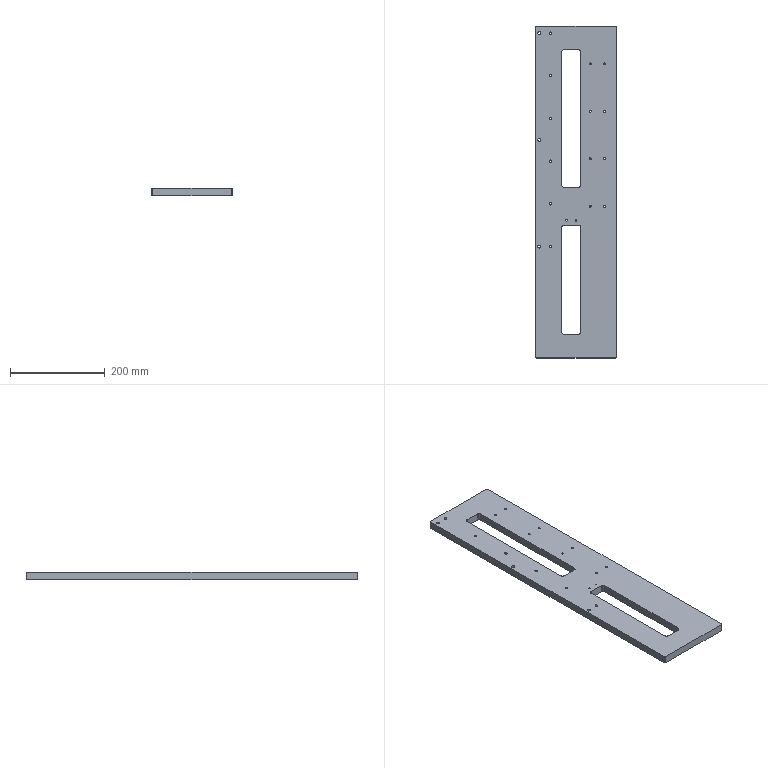Part | STEP file | ASND-0110-LPMF01-028 | 1 solid | 84 faces | box 170 x 700 x 16 mm | volume 1565966 mm3 | cylinder 60 | plane 18 | cone 6 | commonest cylinder face diameters 4.2 x16 10 x16 5 x12 3.3 x10 6.5 x6